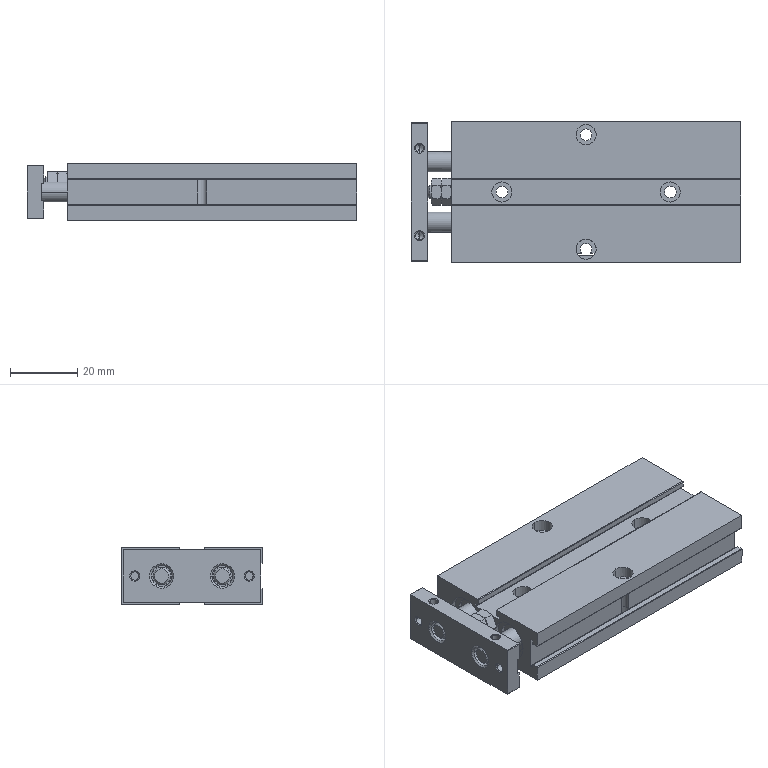Part | SolidWorks | features AEMSimFeature 1 | 2 solids | 277 faces | box 98 x 42 x 17 mm | volume 52480 mm3 | cylinder 109 | plane 104 | cone 64 | commonest cylinder face diameters 0.4 x26 6 x24 2.459 x12 9 x8 10 x8 12 x8